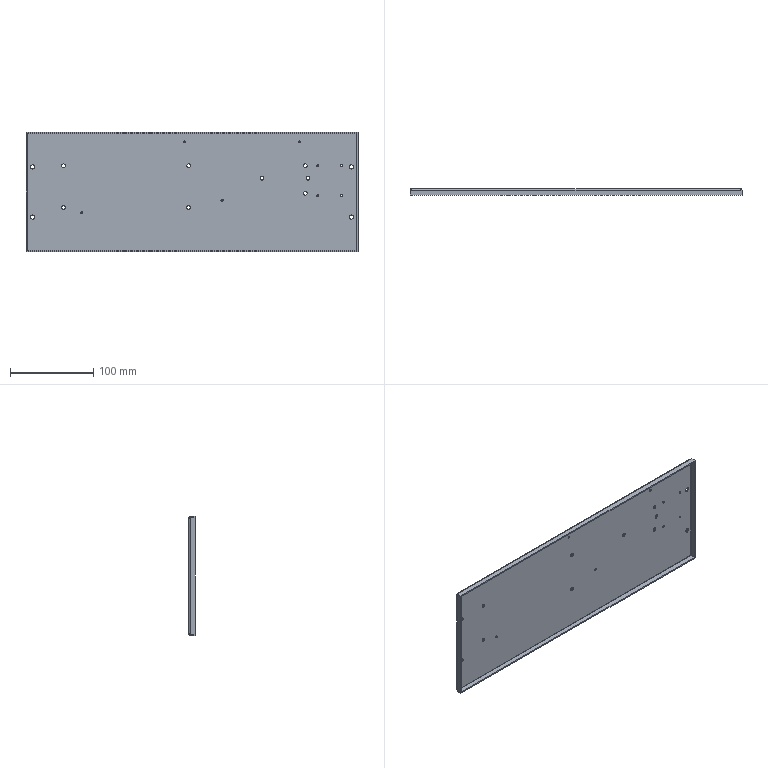Part | STEP file | Power adapter plate 2 | 1 solid | 86 faces | box 398 x 7.5 x 143 mm | volume 93935 mm3 | cylinder 48 | plane 30 | spline 8 | commonest cylinder face diameters 2.5 x16 4.5 x16 5 x8 0.6 x4 3.6 x4